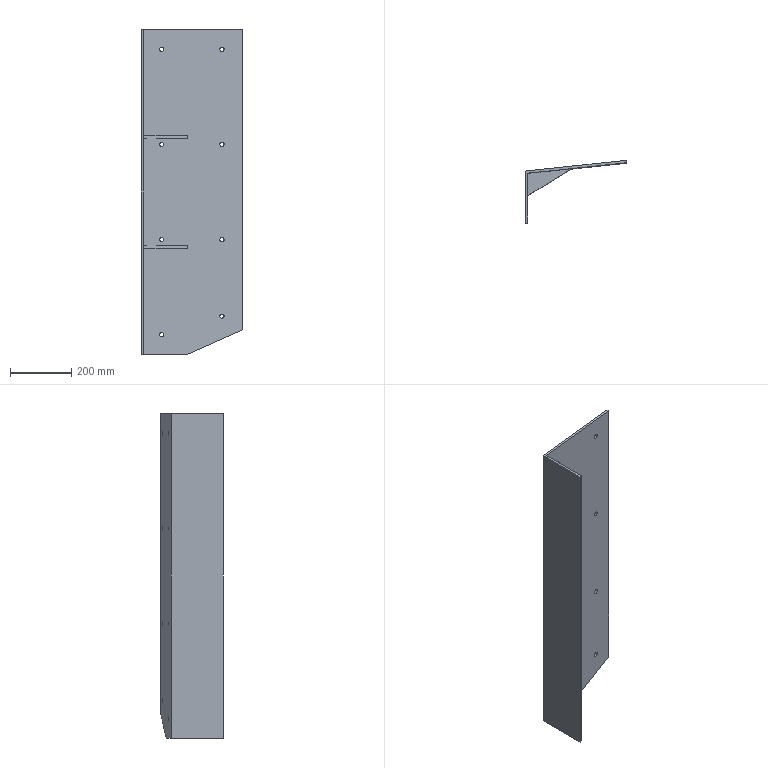Part | STEP file | Bent plate 1_Default<As machined> | 3 solids | 35 faces | box 330 x 204.897 x 1059 mm | volume 4219235 mm3 | plane 19 | cylinder 16 | commonest cylinder face diameters 14 x16